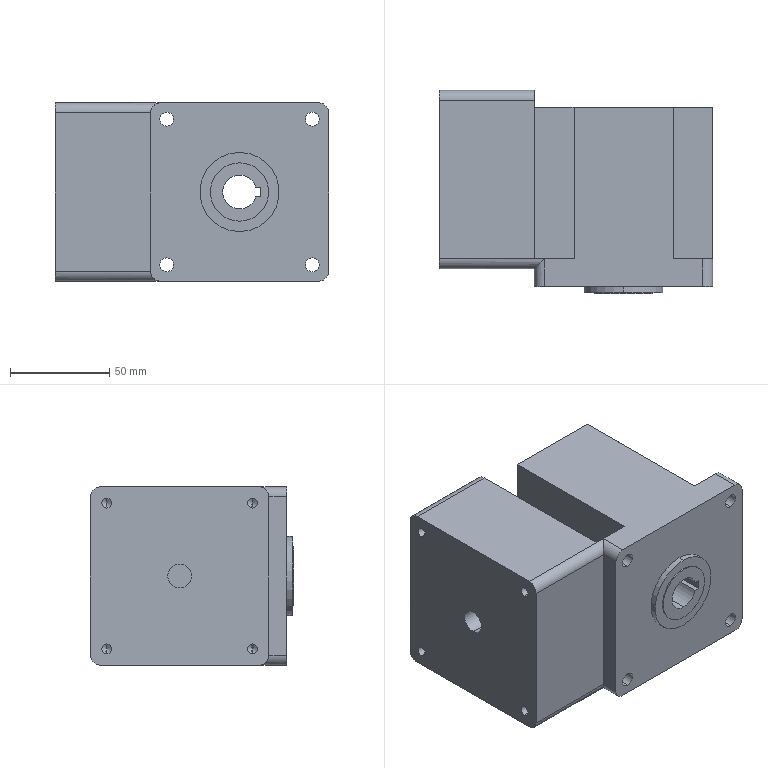Part | SolidWorks | features ICE 10, Fillet 5, CirPattern 3, HoleWzd 2, Chamfer 1, Extrusion 1 | 1 solid | 72 faces | box 138 x 102.5 x 90 mm | volume 974096 mm3 | cylinder 34 | plane 30 | cone 8 | commonest cylinder face diameters 5 x8 7 x8 10 x8 17 x3 12 x2 29.5 x2